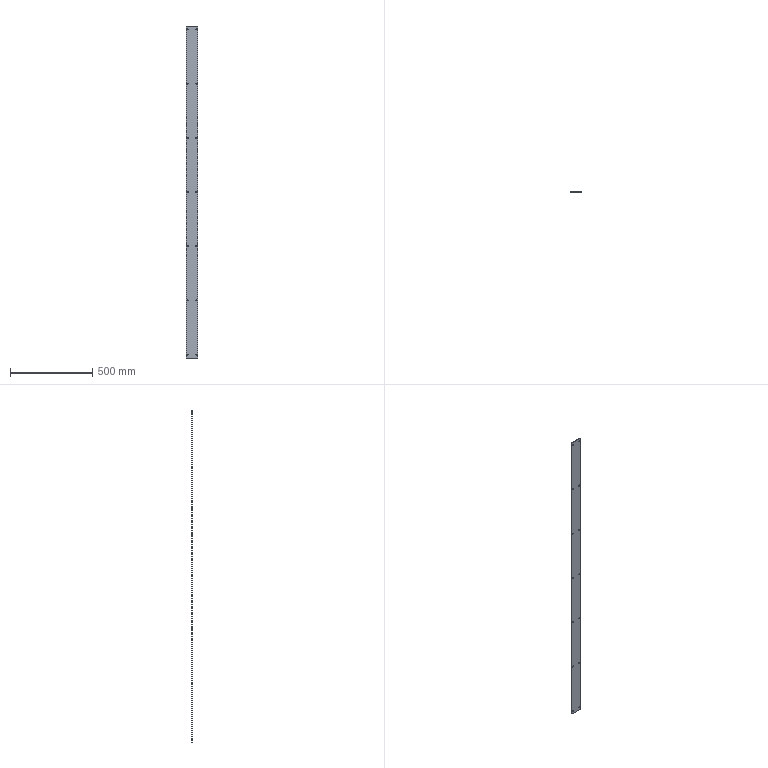Part | 1 solid | 62 faces | box 70 x 1 x 2016 mm | volume 140472 mm3 | plane 34 | cylinder 28 | commonest cylinder face diameters 6 x28